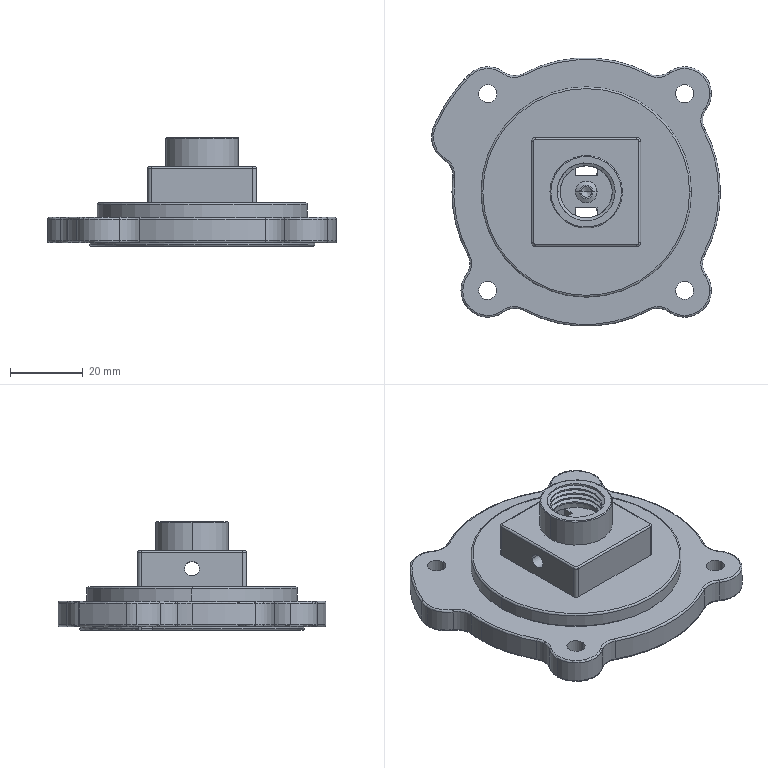Part | SolidWorks | features Fillet 12, ICE 11, Cut 9, HoleWzd 2, MirrorPattern 2, CirPattern 1, Extrusion 1, SweepThread 1 | 1 solid | 308 faces | box 79.627 x 74 x 30 mm | volume 34893 mm3 | cylinder 129 | torus 87 | plane 65 | sphere 16 | spline 7 | cone 4 | commonest cylinder face diameters 0.5 x34 10 x17 16 x10 5 x8 4 x7 1 x6